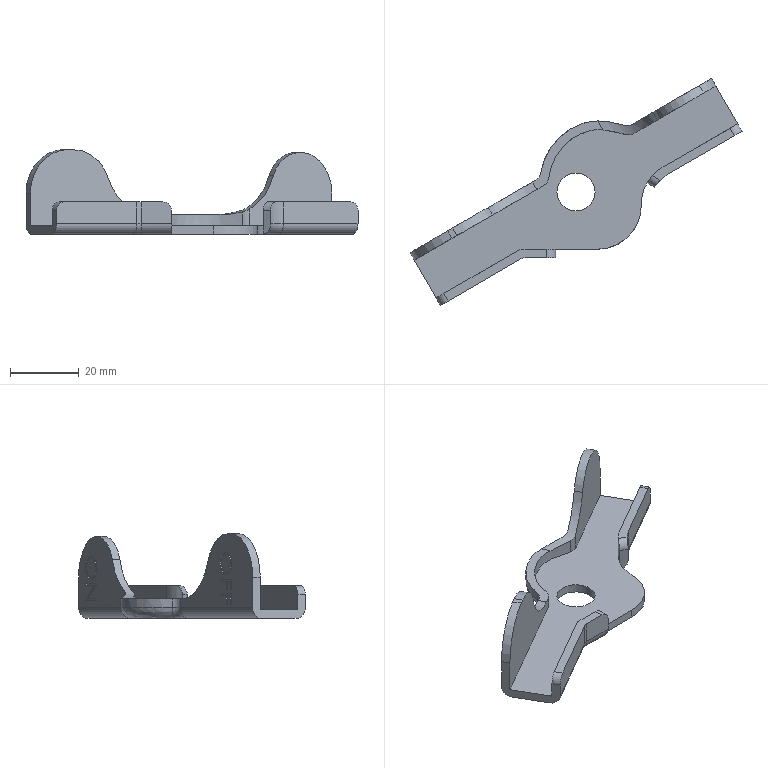Part | SolidWorks | features Fillet 4, ICE 4, Cut 1, FlatPattern 1, SMBaseFlange 1, SheetMetal 1 | 1 solid | 110 faces | box 96.878 x 66.198 x 24.765 mm | volume 9212 mm3 | plane 59 | cylinder 27 | spline 19 | torus 5 | commonest cylinder face diameters 6.35 x9 5.08 x6 25.4 x6 11.112 x2 31.75 x2 19.05 x1